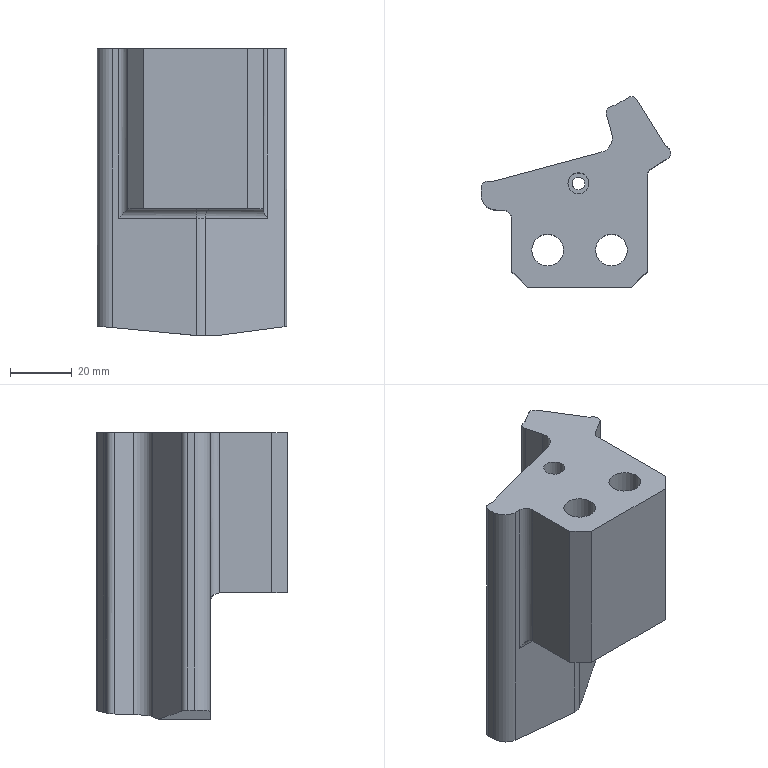Part | NX | features solid 2 | 1 solid | 46 faces | box 61.522 x 61.799 x 92.982 mm | volume 131088 mm3 | cylinder 22 | plane 22 | spline 1 | torus 1 | commonest cylinder face diameters 4 x8 6 x4 10 x4 10.3 x2 17 x2 4.1 x1
STEP:
#1=CARTESIAN_POINT('',(364.121,-6.5,48.));
#2=VERTEX_POINT('',#1);
#3=CARTESIAN_POINT('',(358.971,-6.5,48.));
#4=DIRECTION('',(0.000000738,0.,1.));
#5=DIRECTION('',(1.,0.,-0.000000738));
#6=AXIS2_PLACEMENT_3D('',#3,#4,#5);
#7=CIRCLE('',#6,5.15);
#8=EDGE_CURVE('',#2,#2,#7,.F.);
#9=ORIENTED_EDGE('',*,*,#8,.T.);
#10=EDGE_LOOP('',(#9));
#11=FACE_BOUND('',#10,.T.);
#12=CARTESIAN_POINT('',(353.821,-6.5,78.));
#13=VERTEX_POINT('',#12);
#14=CARTESIAN_POINT('',(358.971,-6.5,78.));
#15=DIRECTION('',(0.,0.,-1.));
#16=DIRECTION('',(-1.,0.,0.));
#17=AXIS2_PLACEMENT_3D('',#14,#15,#16);
#18=CIRCLE('',#17,5.15);
#19=EDGE_CURVE('',#13,#13,#18,.T.);
#20=ORIENTED_EDGE('',*,*,#19,.F.);
#21=EDGE_LOOP('',(#20));
#22=FACE_BOUND('',#21,.T.);
#23=CARTESIAN_POINT('',(358.971,-6.5,54.));
#24=DIRECTION('',(0.000000369,0.000000231,1.));
#25=DIRECTION('',(-1.,0.,0.000000369));
#26=AXIS2_PLACEMENT_3D('',#23,#24,#25);
#27=CYLINDRICAL_SURFACE('',#26,5.15);
#28=ADVANCED_FACE('',(#11,#22),#27,.F.);
#29=ORIENTED_EDGE('',*,*,#8,.F.);
#30=EDGE_LOOP('',(#29));
#31=FACE_BOUND('',#30,.T.);
#32=CARTESIAN_POINT('',(350.471,-6.5,48.));
#33=VERTEX_POINT('',#32);
#34=CARTESIAN_POINT('',(358.971,-6.5,48.));
#35=DIRECTION('',(-0.000000738,0.,-1.));
#36=DIRECTION('',(-1.,0.,0.000000738));
#37=AXIS2_PLACEMENT_3D('',#34,#35,#36);
#38=CIRCLE('',#37,8.5);
#39=EDGE_CURVE('',#33,#33,#38,.T.);
#40=ORIENTED_EDGE('',*,*,#39,.T.);
#41=EDGE_LOOP('',(#40));
#42=FACE_BOUND('',#41,.T.);
#43=CARTESIAN_POINT('',(428.356,-2.,48.));
#44=DIRECTION('',(0.000000738,0.,1.));
#45=DIRECTION('',(1.,0.,-0.000000738));
#46=AXIS2_PLACEMENT_3D('',#43,#44,#45);
#47=PLANE('',#46);
#48=ADVANCED_FACE('',(#31,#42),#47,.F.);
#49=ORIENTED_EDGE('',*,*,#39,.F.);
#50=EDGE_LOOP('',(#49));
#51=FACE_BOUND('',#50,.T.);
#52=CARTESIAN_POINT('',(367.471,-6.5,26.));
#53=VERTEX_POINT('',#52);
#54=CARTESIAN_POINT('',(358.971,-6.5,26.));
#55=DIRECTION('',(0.,0.,1.));
#56=DIRECTION('',(1.,0.,0.));
#57=AXIS2_PLACEMENT_3D('',#54,#55,#56);
#58=CIRCLE('',#57,8.5);
#59=EDGE_CURVE('',#53,#53,#58,.T.);
#60=ORIENTED_EDGE('',*,*,#59,.F.);
#61=EDGE_LOOP('',(#60));
#62=FACE_BOUND('',#61,.T.);
#63=CARTESIAN_POINT('',(358.971,-6.5,19.));
#64=DIRECTION('',(0.000000369,0.000000231,1.));
#65=DIRECTION('',(-1.,0.,0.000000369));
#66=AXIS2_PLACEMENT_3D('',#63,#64,#65);
#67=CYLINDRICAL_SURFACE('',#66,8.5);
#68=ADVANCED_FACE('',(#51,#62),#67,.F.);
#69=CARTESIAN_POINT('',(348.499,17.238,-14.982));
#70=VERTEX_POINT('',#69);
#71=CARTESIAN_POINT('',(348.499,13.166,-14.982));
#72=VERTEX_POINT('',#71);
#73=CARTESIAN_POINT('',(348.26,15.202,-14.982));
#74=DIRECTION('',(-0.000000369,-0.000000231,-1.));
#75=DIRECTION('',(-1.,0.,0.000000369));
#76=AXIS2_PLACEMENT_3D('',#73,#74,#75);
#77=CIRCLE('',#76,2.05);
#78=EDGE_CURVE('',#70,#72,#77,.T.);
#79=ORIENTED_EDGE('',*,*,#78,.F.);
#80=CARTESIAN_POINT('',(348.499,21.837,-14.982));
#81=VERTEX_POINT('',#80);
#82=CARTESIAN_POINT('',(348.499,13.942,-14.982));
#83=DIRECTION('',(0.,1.,-0.000000231));
#84=VECTOR('',#83,1000.);
#85=LINE('',#82,#84);
#86=EDGE_CURVE('',#70,#81,#85,.T.);
#87=ORIENTED_EDGE('',*,*,#86,.T.);
#88=CARTESIAN_POINT('',(355.956,9.904,-14.982));
#89=VERTEX_POINT('',#88);
#90=CARTESIAN_POINT('',(353.665,13.57,-14.982));
#91=DIRECTION('',(0.5299,-0.848,0.));
#92=VECTOR('',#91,1000.);
#93=LINE('',#90,#92);
#94=EDGE_CURVE('',#81,#89,#93,.T.);
#95=ORIENTED_EDGE('',*,*,#94,.T.);
#96=CARTESIAN_POINT('',(351.724,7.26,-14.982));
#97=VERTEX_POINT('',#96);
#98=CARTESIAN_POINT('',(347.525,4.636,-14.982));
#99=DIRECTION('',(0.848,0.5299,-0.000000435));
#100=VECTOR('',#99,1000.);
#101=LINE('',#98,#100);
#102=EDGE_CURVE('',#97,#89,#101,.T.);
#103=ORIENTED_EDGE('',*,*,#102,.F.);
#104=CARTESIAN_POINT('',(349.074,6.5,-14.982));
#105=VERTEX_POINT('',#104);
#106=CARTESIAN_POINT('',(349.074,11.5,-14.982));
#107=DIRECTION('',(-0.000000369,-0.000000231,-1.));
#108=DIRECTION('',(-1.,0.,0.000000369));
#109=AXIS2_PLACEMENT_3D('',#106,#107,#108);
#110=CIRCLE('',#109,5.);
#111=EDGE_CURVE('',#97,#105,#110,.T.);
#112=ORIENTED_EDGE('',*,*,#111,.T.);
#113=CARTESIAN_POINT('',(348.499,6.5,-14.982));
#114=VERTEX_POINT('',#113);
#115=CARTESIAN_POINT('',(297.,6.5,-14.982));
#116=DIRECTION('',(1.,0.,-0.000000369));
#117=VECTOR('',#116,1000.);
#118=LINE('',#115,#117);
#119=EDGE_CURVE('',#114,#105,#118,.T.);
#120=ORIENTED_EDGE('',*,*,#119,.F.);
#121=CARTESIAN_POINT('',(348.499,13.942,-14.982));
#122=DIRECTION('',(0.,1.,-0.000000231));
#123=VECTOR('',#122,1000.);
#124=LINE('',#121,#123);
#125=EDGE_CURVE('',#114,#72,#124,.T.);
#126=ORIENTED_EDGE('',*,*,#125,.T.);
#127=EDGE_LOOP('',(#79,#87,#95,#103,#112,#120,#126));
#128=FACE_BOUND('',#127,.T.);
#129=CARTESIAN_POINT('',(294.129,90.087,-14.982));
#130=DIRECTION('',(-0.000000369,-0.000000231,-1.));
#131=DIRECTION('',(-1.,0.,0.000000369));
#132=AXIS2_PLACEMENT_3D('',#129,#130,#131);
#133=PLANE('',#132);
#134=ADVANCED_FACE('',(#128),#133,.T.);
#135=CARTESIAN_POINT('',(343.413,-6.5,48.));
#136=VERTEX_POINT('',#135);
#137=CARTESIAN_POINT('',(338.263,-6.5,48.));
#138=DIRECTION('',(0.,0.,1.));
#139=DIRECTION('',(1.,0.,0.));
#140=AXIS2_PLACEMENT_3D('',#137,#138,#139);
#141=CIRCLE('',#140,5.15);
#142=EDGE_CURVE('',#136,#136,#141,.F.);
#143=ORIENTED_EDGE('',*,*,#142,.F.);
#144=EDGE_LOOP('',(#143));
#145=FACE_BOUND('',#144,.T.);
#146=CARTESIAN_POINT('',(346.763,-6.5,48.));
#147=VERTEX_POINT('',#146);
#148=CARTESIAN_POINT('',(338.263,-6.5,48.));
#149=DIRECTION('',(0.,0.,1.));
#150=DIRECTION('',(1.,0.,0.));
#151=AXIS2_PLACEMENT_3D('',#148,#149,#150);
#152=CIRCLE('',#151,8.5);
#153=EDGE_CURVE('',#147,#147,#152,.F.);
#154=ORIENTED_EDGE('',*,*,#153,.T.);
#155=EDGE_LOOP('',(#154));
#156=FACE_BOUND('',#155,.T.);
#157=CARTESIAN_POINT('',(268.879,-2.,48.));
#158=DIRECTION('',(0.,0.,1.));
#159=DIRECTION('',(-1.,0.,0.));
#160=AXIS2_PLACEMENT_3D('',#157,#158,#159);
#161=PLANE('',#160);
#162=ADVANCED_FACE('',(#145,#156),#161,.F.);
#163=CARTESIAN_POINT('',(316.719,11.5,-11.955));
#164=VERTEX_POINT('',#163);
#165=CARTESIAN_POINT('',(316.719,11.5,78.));
#166=VERTEX_POINT('',#165);
#167=CARTESIAN_POINT('',(316.719,11.5,-8.));
#168=DIRECTION('',(0.000000369,0.000000231,1.));
#169=VECTOR('',#168,1000.);
#170=LINE('',#167,#169);
#171=EDGE_CURVE('',#164,#166,#170,.T.);
#172=ORIENTED_EDGE('',*,*,#171,.F.);
#173=CARTESIAN_POINT('',(321.719,6.5,-12.431));
#174=VERTEX_POINT('',#173);
#175=CARTESIAN_POINT('',(321.719,11.5,-12.431));
#176=DIRECTION('',(-0.09481,-0.00000023,-0.9955));
#177=DIRECTION('',(-0.9955,0.000000022,0.09481));
#178=AXIS2_PLACEMENT_3D('',#175,#176,#177);
#179=ELLIPSE('',#178,5.023,5.);
#180=EDGE_CURVE('',#164,#174,#179,.F.);
#181=ORIENTED_EDGE('',*,*,#180,.T.);
#182=CARTESIAN_POINT('',(321.719,6.5,78.));
#183=VERTEX_POINT('',#182);
#184=CARTESIAN_POINT('',(321.719,6.5,-8.));
#185=DIRECTION('',(0.000000369,0.000000231,1.));
#186=VECTOR('',#185,1000.);
#187=LINE('',#184,#186);
#188=EDGE_CURVE('',#174,#183,#187,.T.);
#189=ORIENTED_EDGE('',*,*,#188,.T.);
#190=CARTESIAN_POINT('',(321.719,11.5,78.));
#191=DIRECTION('',(0.,0.,-1.));
#192=DIRECTION('',(-1.,0.,0.));
#193=AXIS2_PLACEMENT_3D('',#190,#191,#192);
#194=CIRCLE('',#193,5.);
#195=EDGE_CURVE('',#183,#166,#194,.T.);
#196=ORIENTED_EDGE('',*,*,#195,.T.);
#197=EDGE_LOOP('',(#172,#181,#189,#196));
#198=FACE_BOUND('',#197,.T.);
#199=CARTESIAN_POINT('',(321.719,11.5,-8.));
#200=DIRECTION('',(0.000000369,0.000000231,1.));
#201=DIRECTION('',(1.,0.,-0.000000369));
#202=AXIS2_PLACEMENT_3D('',#199,#200,#201);
#203=CYLINDRICAL_SURFACE('',#202,5.);
#204=ADVANCED_FACE('',(#198),#203,.T.);
#205=CARTESIAN_POINT('',(316.719,13.767,-11.955));
#206=VERTEX_POINT('',#205);
#207=CARTESIAN_POINT('',(316.719,13.767,78.));
#208=VERTEX_POINT('',#207);
#209=CARTESIAN_POINT('',(316.719,13.767,-8.));
#210=DIRECTION('',(0.000000369,0.000000231,1.));
#211=VECTOR('',#210,1000.);
#212=LINE('',#209,#211);
#213=EDGE_CURVE('',#206,#208,#212,.T.);
#214=ORIENTED_EDGE('',*,*,#213,.F.);
#215=CARTESIAN_POINT('',(316.719,90.087,-11.955));
#216=DIRECTION('',(0.,-1.,0.000000231));
#217=VECTOR('',#216,1000.);
#218=LINE('',#215,#217);
#219=EDGE_CURVE('',#206,#164,#218,.T.);
#220=ORIENTED_EDGE('',*,*,#219,.T.);
#221=ORIENTED_EDGE('',*,*,#171,.T.);
#222=CARTESIAN_POINT('',(316.719,89.912,78.));
#223=DIRECTION('',(0.,1.,0.));
#224=VECTOR('',#223,1000.);
#225=LINE('',#222,#224);
#226=EDGE_CURVE('',#166,#208,#225,.T.);
#227=ORIENTED_EDGE('',*,*,#226,.T.);
#228=EDGE_LOOP('',(#214,#220,#221,#227));
#229=FACE_BOUND('',#228,.T.);
#230=CARTESIAN_POINT('',(316.719,89.912,-8.));
#231=DIRECTION('',(1.,0.,-0.000000369));
#232=DIRECTION('',(-0.000000369,0.,-1.));
#233=AXIS2_PLACEMENT_3D('',#230,#231,#232);
#234=PLANE('',#233);
#235=ADVANCED_FACE('',(#229),#234,.F.);
#236=CARTESIAN_POINT('',(318.201,15.698,-12.096));
#237=VERTEX_POINT('',#236);
#238=CARTESIAN_POINT('',(318.201,15.698,78.));
#239=VERTEX_POINT('',#238);
#240=CARTESIAN_POINT('',(318.201,15.698,-8.));
#241=DIRECTION('',(0.000000369,0.000000231,1.));
#242=VECTOR('',#241,1000.);
#243=LINE('',#240,#242);
#244=EDGE_CURVE('',#237,#239,#243,.T.);
#245=ORIENTED_EDGE('',*,*,#244,.F.);
#246=CARTESIAN_POINT('',(318.719,13.767,-12.145));
#247=DIRECTION('',(-0.09481,-0.00000023,-0.9955));
#248=DIRECTION('',(-0.9955,0.000000022,0.09481));
#249=AXIS2_PLACEMENT_3D('',#246,#247,#248);
#250=ELLIPSE('',#249,2.009,2.);
#251=EDGE_CURVE('',#237,#206,#250,.F.);
#252=ORIENTED_EDGE('',*,*,#251,.T.);
#253=ORIENTED_EDGE('',*,*,#213,.T.);
#254=CARTESIAN_POINT('',(318.719,13.767,78.));
#255=DIRECTION('',(0.,0.,-1.));
#256=DIRECTION('',(-1.,0.,0.));
#257=AXIS2_PLACEMENT_3D('',#254,#255,#256);
#258=CIRCLE('',#257,2.);
#259=EDGE_CURVE('',#208,#239,#258,.T.);
#260=ORIENTED_EDGE('',*,*,#259,.T.);
#261=EDGE_LOOP('',(#245,#252,#253,#260));
#262=FACE_BOUND('',#261,.T.);
#263=CARTESIAN_POINT('',(318.719,13.767,-8.));
#264=DIRECTION('',(0.000000369,0.000000231,1.));
#265=DIRECTION('',(1.,0.,-0.000000369));
#266=AXIS2_PLACEMENT_3D('',#263,#264,#265);
#267=CYLINDRICAL_SURFACE('',#266,2.);
#268=ADVANCED_FACE('',(#262),#267,.T.);
#269=CARTESIAN_POINT('',(318.626,15.812,-12.137));
#270=VERTEX_POINT('',#269);
#271=CARTESIAN_POINT('',(318.626,15.812,78.));
#272=VERTEX_POINT('',#271);
#273=CARTESIAN_POINT('',(318.626,15.812,-8.));
#274=DIRECTION('',(0.000000369,0.000000231,1.));
#275=VECTOR('',#274,1000.);
#276=LINE('',#273,#275);
#277=EDGE_CURVE('',#270,#272,#276,.T.);
#278=ORIENTED_EDGE('',*,*,#277,.F.);
#279=CARTESIAN_POINT('',(364.928,28.219,-16.546));
#280=DIRECTION('',(-0.9619,-0.2577,0.09161));
#281=VECTOR('',#280,1000.);
#282=LINE('',#279,#281);
#283=EDGE_CURVE('',#270,#237,#282,.T.);
#284=ORIENTED_EDGE('',*,*,#283,.T.);
#285=ORIENTED_EDGE('',*,*,#244,.T.);
#286=CARTESIAN_POINT('',(303.806,11.841,78.));
#287=DIRECTION('',(0.9659,0.2588,0.));
#288=VECTOR('',#287,1000.);
#289=LINE('',#286,#288);
#290=EDGE_CURVE('',#239,#272,#289,.T.);
#291=ORIENTED_EDGE('',*,*,#290,.T.);
#292=EDGE_LOOP('',(#278,#284,#285,#291));
#293=FACE_BOUND('',#292,.T.);
#294=CARTESIAN_POINT('',(303.806,11.841,-8.));
#295=DIRECTION('',(0.2588,-0.9659,0.000000127));
#296=DIRECTION('',(0.9659,0.2588,0.));
#297=AXIS2_PLACEMENT_3D('',#294,#295,#296);
#298=PLANE('',#297);
#299=ADVANCED_FACE('',(#293),#298,.F.);
#300=CARTESIAN_POINT('',(319.626,15.821,-12.232));
#301=VERTEX_POINT('',#300);
#302=CARTESIAN_POINT('',(319.626,15.821,78.));
#303=VERTEX_POINT('',#302);
#304=CARTESIAN_POINT('',(319.626,15.821,-8.));
#305=DIRECTION('',(0.000000369,0.000000231,1.));
#306=VECTOR('',#305,1000.);
#307=LINE('',#304,#306);
#308=EDGE_CURVE('',#301,#303,#307,.T.);
#309=ORIENTED_EDGE('',*,*,#308,.F.);
#310=CARTESIAN_POINT('',(319.143,13.88,-12.186));
#311=DIRECTION('',(-0.09481,-0.00000023,-0.9955));
#312=DIRECTION('',(-0.9955,0.000000022,0.09481));
#313=AXIS2_PLACEMENT_3D('',#310,#311,#312);
#314=ELLIPSE('',#313,2.009,2.);
#315=EDGE_CURVE('',#301,#270,#314,.F.);
#316=ORIENTED_EDGE('',*,*,#315,.T.);
#317=ORIENTED_EDGE('',*,*,#277,.T.);
#318=CARTESIAN_POINT('',(319.143,13.88,78.));
#319=DIRECTION('',(0.,0.,-1.));
#320=DIRECTION('',(-1.,0.,0.));
#321=AXIS2_PLACEMENT_3D('',#318,#319,#320);
#322=CIRCLE('',#321,2.);
#323=EDGE_CURVE('',#272,#303,#322,.T.);
#324=ORIENTED_EDGE('',*,*,#323,.T.);
#325=EDGE_LOOP('',(#309,#316,#317,#324));
#326=FACE_BOUND('',#325,.T.);
#327=CARTESIAN_POINT('',(319.143,13.88,-8.));
#328=DIRECTION('',(0.000000369,0.000000231,1.));
#329=DIRECTION('',(1.,0.,-0.000000369));
#330=AXIS2_PLACEMENT_3D('',#327,#328,#329);
#331=CYLINDRICAL_SURFACE('',#330,2.);
#332=ADVANCED_FACE('',(#326),#331,.T.);
#333=CARTESIAN_POINT('',(320.626,15.83,-12.327));
#334=VERTEX_POINT('',#333);
#335=CARTESIAN_POINT('',(320.626,15.831,78.));
#336=VERTEX_POINT('',#335);
#337=CARTESIAN_POINT('',(320.626,15.83,-8.));
#338=DIRECTION('',(0.000000369,0.000000231,1.));
#339=VECTOR('',#338,1000.);
#340=LINE('',#337,#339);
#341=EDGE_CURVE('',#334,#336,#340,.T.);
#342=ORIENTED_EDGE('',*,*,#341,.F.);
#343=CARTESIAN_POINT('',(320.108,17.762,-12.278));
#344=DIRECTION('',(-0.09481,-0.00000023,-0.9955));
#345=DIRECTION('',(-0.9955,0.000000022,0.09481));
#346=AXIS2_PLACEMENT_3D('',#343,#344,#345);
#347=ELLIPSE('',#346,2.009,2.);
#348=EDGE_CURVE('',#334,#301,#347,.T.);
#349=ORIENTED_EDGE('',*,*,#348,.T.);
#350=ORIENTED_EDGE('',*,*,#308,.T.);
#351=CARTESIAN_POINT('',(320.108,17.762,78.));
#352=DIRECTION('',(0.,0.,-1.));
#353=DIRECTION('',(-1.,0.,0.));
#354=AXIS2_PLACEMENT_3D('',#351,#352,#353);
#355=CIRCLE('',#354,2.);
#356=EDGE_CURVE('',#303,#336,#355,.F.);
#357=ORIENTED_EDGE('',*,*,#356,.T.);
#358=EDGE_LOOP('',(#342,#349,#350,#357));
#359=FACE_BOUND('',#358,.T.);
#360=CARTESIAN_POINT('',(320.108,17.762,-8.));
#361=DIRECTION('',(0.000000369,0.000000231,1.));
#362=DIRECTION('',(1.,0.,-0.000000369));
#363=AXIS2_PLACEMENT_3D('',#360,#361,#362);
#364=CYLINDRICAL_SURFACE('',#363,2.);
#365=ADVANCED_FACE('',(#359),#364,.F.);
#366=CARTESIAN_POINT('',(355.551,25.189,-14.12));
#367=VERTEX_POINT('',#366);
#368=CARTESIAN_POINT('',(348.08,23.187,-14.942));
#369=VERTEX_POINT('',#368);
#370=CARTESIAN_POINT('',(323.92,16.713,-17.599));
#371=DIRECTION('',(-0.9605,-0.2574,-0.1057));
#372=VECTOR('',#371,1000.);
#373=LINE('',#370,#372);
#374=EDGE_CURVE('',#367,#369,#373,.T.);
#375=ORIENTED_EDGE('',*,*,#374,.T.);
#376=CARTESIAN_POINT('',(365.056,27.736,-16.559));
#377=DIRECTION('',(-0.9619,-0.2577,0.09161));
#378=VECTOR('',#377,1000.);
#379=LINE('',#376,#378);
#380=EDGE_CURVE('',#369,#334,#379,.T.);
#381=ORIENTED_EDGE('',*,*,#380,.T.);
#382=ORIENTED_EDGE('',*,*,#341,.T.);
#383=CARTESIAN_POINT('',(355.551,25.189,78.));
#384=VERTEX_POINT('',#383);
#385=CARTESIAN_POINT('',(320.626,15.831,78.));
#386=DIRECTION('',(0.9659,0.2588,0.));
#387=VECTOR('',#386,1000.);
#388=LINE('',#385,#387);
#389=EDGE_CURVE('',#336,#384,#388,.T.);
#390=ORIENTED_EDGE('',*,*,#389,.T.);
#391=CARTESIAN_POINT('',(355.551,25.189,-8.));
#392=DIRECTION('',(0.000000369,0.000000231,1.));
#393=VECTOR('',#392,1000.);
#394=LINE('',#391,#393);
#395=EDGE_CURVE('',#367,#384,#394,.T.);
#396=ORIENTED_EDGE('',*,*,#395,.F.);
#397=EDGE_LOOP('',(#375,#381,#382,#390,#396));
#398=FACE_BOUND('',#397,.T.);
#399=CARTESIAN_POINT('',(320.626,15.83,-8.));
#400=DIRECTION('',(0.2588,-0.9659,0.000000127));
#401=DIRECTION('',(0.9659,0.2588,0.));
#402=AXIS2_PLACEMENT_3D('',#399,#400,#401);
#403=PLANE('',#402);
#404=ADVANCED_FACE('',(#398),#403,.F.);
#405=CARTESIAN_POINT('',(359.061,31.404,-13.423));
#406=VERTEX_POINT('',#405);
#407=CARTESIAN_POINT('',(359.061,31.404,78.));
#408=VERTEX_POINT('',#407);
#409=CARTESIAN_POINT('',(359.061,31.404,-8.));
#410=DIRECTION('',(0.000000369,0.000000231,1.));
#411=VECTOR('',#410,1000.);
#412=LINE('',#409,#411);
#413=EDGE_CURVE('',#406,#408,#412,.T.);
#414=ORIENTED_EDGE('',*,*,#413,.F.);
#415=CARTESIAN_POINT('',(354.257,30.018,-13.957));
#416=DIRECTION('',(0.09365,0.05852,-0.9939));
#417=DIRECTION('',(0.8429,0.5267,0.1104));
#418=AXIS2_PLACEMENT_3D('',#415,#416,#417);
#419=ELLIPSE('',#418,5.031,5.);
#420=EDGE_CURVE('',#406,#367,#419,.T.);
#421=ORIENTED_EDGE('',*,*,#420,.T.);
#422=ORIENTED_EDGE('',*,*,#395,.T.);
#423=CARTESIAN_POINT('',(354.257,30.018,78.));
#424=DIRECTION('',(0.,0.,-1.));
#425=DIRECTION('',(-1.,0.,0.));
#426=AXIS2_PLACEMENT_3D('',#423,#424,#425);
#427=CIRCLE('',#426,5.);
#428=EDGE_CURVE('',#384,#408,#427,.F.);
#429=ORIENTED_EDGE('',*,*,#428,.T.);
#430=EDGE_LOOP('',(#414,#421,#422,#429));
#431=FACE_BOUND('',#430,.T.);
#432=CARTESIAN_POINT('',(354.257,30.018,-8.));
#433=DIRECTION('',(0.000000369,0.000000231,1.));
#434=DIRECTION('',(1.,0.,-0.000000369));
#435=AXIS2_PLACEMENT_3D('',#432,#433,#434);
#436=CYLINDRICAL_SURFACE('',#435,5.);
#437=ADVANCED_FACE('',(#431),#436,.F.);
#438=CARTESIAN_POINT('',(357.296,37.575,78.));
#439=VERTEX_POINT('',#438);
#440=CARTESIAN_POINT('',(357.296,37.575,-13.226));
#441=VERTEX_POINT('',#440);
#442=CARTESIAN_POINT('',(357.296,37.575,82.));
#443=DIRECTION('',(0.000000369,0.000000231,1.));
#444=VECTOR('',#443,1000.);
#445=LINE('',#442,#444);
#446=EDGE_CURVE('',#439,#441,#445,.F.);
#447=ORIENTED_EDGE('',*,*,#446,.T.);
#448=CARTESIAN_POINT('',(357.296,37.575,-13.226));
#449=CARTESIAN_POINT('',(357.879,35.516,-13.292));
#450=CARTESIAN_POINT('',(358.468,33.46,-13.358));
#451=CARTESIAN_POINT('',(359.061,31.404,-13.423));
#452=B_SPLINE_CURVE_WITH_KNOTS('',3,(#448,#449,#450,#451),.UNSPECIFIED.,.F.,.F.,(4,4),(0.,0.006421),.UNSPECIFIED.);
#453=EDGE_CURVE('',#441,#406,#452,.T.);
#454=ORIENTED_EDGE('',*,*,#453,.T.);
#455=ORIENTED_EDGE('',*,*,#413,.T.);
#456=CARTESIAN_POINT('',(359.061,31.404,78.));
#457=CARTESIAN_POINT('',(358.469,33.46,78.));
#458=CARTESIAN_POINT('',(357.879,35.516,78.));
#459=CARTESIAN_POINT('',(357.296,37.575,78.));
#460=B_SPLINE_CURVE_WITH_KNOTS('',3,(#456,#457,#458,#459),.UNSPECIFIED.,.F.,.F.,(4,4),(0.,0.006418),.UNSPECIFIED.);
#461=EDGE_CURVE('',#408,#439,#460,.T.);
#462=ORIENTED_EDGE('',*,*,#461,.T.);
#463=EDGE_LOOP('',(#447,#454,#455,#462));
#464=FACE_BOUND('',#463,.T.);
#465=CARTESIAN_POINT('',(359.061,31.404,-13.972));
#466=CARTESIAN_POINT('',(359.061,31.404,78.));
#467=CARTESIAN_POINT('',(358.468,33.46,-13.972));
#468=CARTESIAN_POINT('',(358.469,33.46,78.));
#469=CARTESIAN_POINT('',(357.879,35.516,-13.972));
#470=CARTESIAN_POINT('',(357.879,35.516,78.));
#471=CARTESIAN_POINT('',(357.296,37.575,-13.972));
#472=CARTESIAN_POINT('',(357.296,37.575,78.));
#473=B_SPLINE_SURFACE_WITH_KNOTS('',3,1,((#465,#466),(#467,#468),(#469,#470),(#471,#472)),.SURF_OF_LINEAR_EXTRUSION.,.F.,.F.,.F.,(4,4),(2,2),(-0.02584,0.4694),(0.,1.),.PIECEWISE_BEZIER_KNOTS.);
#474=ADVANCED_FACE('',(#464),#473,.F.);
#475=CARTESIAN_POINT('',(358.674,40.044,-12.951));
#476=VERTEX_POINT('',#475);
#477=CARTESIAN_POINT('',(358.674,40.044,78.));
#478=VERTEX_POINT('',#477);
#479=CARTESIAN_POINT('',(358.674,40.044,82.));
#480=DIRECTION('',(-0.000000369,-0.000000231,-1.));
#481=VECTOR('',#480,1000.);
#482=LINE('',#479,#481);
#483=EDGE_CURVE('',#476,#478,#482,.F.);
#484=ORIENTED_EDGE('',*,*,#483,.F.);
#485=CARTESIAN_POINT('',(359.22,38.12,-13.013));
#486=DIRECTION('',(0.09365,0.05852,-0.9939));
#487=DIRECTION('',(0.8429,0.5267,0.1104));
#488=AXIS2_PLACEMENT_3D('',#485,#486,#487);
#489=ELLIPSE('',#488,2.012,2.);
#490=EDGE_CURVE('',#476,#441,#489,.F.);
#491=ORIENTED_EDGE('',*,*,#490,.T.);
#492=ORIENTED_EDGE('',*,*,#446,.F.);
#493=CARTESIAN_POINT('',(359.22,38.12,78.));
#494=DIRECTION('',(0.,0.,-1.));
#495=DIRECTION('',(-1.,0.,0.));
#496=AXIS2_PLACEMENT_3D('',#493,#494,#495);
#497=CIRCLE('',#496,2.);
#498=EDGE_CURVE('',#478,#439,#497,.F.);
#499=ORIENTED_EDGE('',*,*,#498,.F.);
#500=EDGE_LOOP('',(#484,#491,#492,#499));
#501=FACE_BOUND('',#500,.T.);
#502=CARTESIAN_POINT('',(359.22,38.12,37.));
#503=DIRECTION('',(0.000000369,0.000000231,1.));
#504=DIRECTION('',(1.,0.,-0.000000369));
#505=AXIS2_PLACEMENT_3D('',#502,#503,#504);
#506=CYLINDRICAL_SURFACE('',#505,2.);
#507=ADVANCED_FACE('',(#501),#506,.T.);
#508=CARTESIAN_POINT('',(359.771,40.356,78.));
#509=VERTEX_POINT('',#508);
#510=CARTESIAN_POINT('',(359.771,40.356,-12.829));
#511=VERTEX_POINT('',#510);
#512=CARTESIAN_POINT('',(359.771,40.356,-8.));
#513=DIRECTION('',(0.000000369,0.000000231,1.));
#514=VECTOR('',#513,1000.);
#515=LINE('',#512,#514);
#516=EDGE_CURVE('',#509,#511,#515,.F.);
#517=ORIENTED_EDGE('',*,*,#516,.T.);
#518=CARTESIAN_POINT('',(312.387,26.918,-18.085));
#519=DIRECTION('',(-0.9566,-0.2713,-0.1061));
#520=VECTOR('',#519,1000.);
#521=LINE('',#518,#520);
#522=EDGE_CURVE('',#511,#476,#521,.T.);
#523=ORIENTED_EDGE('',*,*,#522,.T.);
#524=ORIENTED_EDGE('',*,*,#483,.T.);
#525=CARTESIAN_POINT('',(311.762,26.741,78.));
#526=DIRECTION('',(-0.9621,-0.2728,0.));
#527=VECTOR('',#526,1000.);
#528=LINE('',#525,#527);
#529=EDGE_CURVE('',#509,#478,#528,.T.);
#530=ORIENTED_EDGE('',*,*,#529,.F.);
#531=EDGE_LOOP('',(#517,#523,#524,#530));
#532=FACE_BOUND('',#531,.T.);
#533=CARTESIAN_POINT('',(311.762,26.741,-8.));
#534=DIRECTION('',(-0.2728,0.9621,-0.000000121));
#535=DIRECTION('',(-0.9621,-0.2728,0.));
#536=AXIS2_PLACEMENT_3D('',#533,#534,#535);
#537=PLANE('',#536);
#538=ADVANCED_FACE('',(#532),#537,.T.);
#539=CARTESIAN_POINT('',(361.056,40.926,-12.675));
#540=VERTEX_POINT('',#539);
#541=CARTESIAN_POINT('',(361.057,40.926,78.));
#542=VERTEX_POINT('',#541);
#543=CARTESIAN_POINT('',(361.057,40.926,82.));
#544=DIRECTION('',(0.000000369,0.000000231,1.));
#545=VECTOR('',#544,1000.);
#546=LINE('',#543,#545);
#547=EDGE_CURVE('',#540,#542,#546,.T.);
#548=ORIENTED_EDGE('',*,*,#547,.F.);
#549=CARTESIAN_POINT('',(358.407,45.166,-12.675));
#550=DIRECTION('',(0.09365,0.05852,-0.9939));
#551=DIRECTION('',(-0.8429,-0.5267,-0.1104));
#552=AXIS2_PLACEMENT_3D('',#549,#550,#551);
#553=ELLIPSE('',#552,5.031,5.);
#554=EDGE_CURVE('',#540,#511,#553,.T.);
#555=ORIENTED_EDGE('',*,*,#554,.T.);
#556=ORIENTED_EDGE('',*,*,#516,.F.);
#557=CARTESIAN_POINT('',(358.407,45.166,78.));
#558=DIRECTION('',(0.,0.,-1.));
#559=DIRECTION('',(-1.,0.,0.));
#560=AXIS2_PLACEMENT_3D('',#557,#558,#559);
#561=CIRCLE('',#560,5.);
#562=EDGE_CURVE('',#542,#509,#561,.T.);
#563=ORIENTED_EDGE('',*,*,#562,.F.);
#564=EDGE_LOOP('',(#548,#555,#556,#563));
#565=FACE_BOUND('',#564,.T.);
#566=CARTESIAN_POINT('',(358.407,45.166,-8.));
#567=DIRECTION('',(-0.000000369,-0.000000231,-1.));
#568=DIRECTION('',(-1.,0.,0.000000369));
#569=AXIS2_PLACEMENT_3D('',#566,#567,#568);
#570=CYLINDRICAL_SURFACE('',#569,5.);
#571=ADVANCED_FACE('',(#565),#570,.F.);
#572=CARTESIAN_POINT('',(364.368,42.995,78.));
#573=VERTEX_POINT('',#572);
#574=CARTESIAN_POINT('',(364.368,42.995,-12.241));
#575=VERTEX_POINT('',#574);
#576=CARTESIAN_POINT('',(364.368,42.995,-8.));
#577=DIRECTION('',(-0.000000369,-0.000000231,-1.));
#578=VECTOR('',#577,1000.);
#579=LINE('',#576,#578);
#580=EDGE_CURVE('',#573,#575,#579,.T.);
#581=ORIENTED_EDGE('',*,*,#580,.T.);
#582=CARTESIAN_POINT('',(335.119,24.718,-16.073));
#583=DIRECTION('',(-0.8429,-0.5267,-0.1104));
#584=VECTOR('',#583,1000.);
#585=LINE('',#582,#584);
#586=EDGE_CURVE('',#575,#540,#585,.T.);
#587=ORIENTED_EDGE('',*,*,#586,.T.);
#588=ORIENTED_EDGE('',*,*,#547,.T.);
#589=CARTESIAN_POINT('',(334.735,24.478,78.));
#590=DIRECTION('',(-0.848,-0.5299,0.));
#591=VECTOR('',#590,1000.);
#592=LINE('',#589,#591);
#593=EDGE_CURVE('',#573,#542,#592,.T.);
#594=ORIENTED_EDGE('',*,*,#593,.F.);
#595=EDGE_LOOP('',(#581,#587,#588,#594));
#596=FACE_BOUND('',#595,.T.);
#597=CARTESIAN_POINT('',(334.735,24.478,-8.));
#598=DIRECTION('',(-0.5299,0.848,0.));
#599=DIRECTION('',(-0.848,-0.5299,0.));
#600=AXIS2_PLACEMENT_3D('',#597,#598,#599);
#601=PLANE('',#600);
#602=ADVANCED_FACE('',(#596),#601,.T.);
#603=CARTESIAN_POINT('',(367.124,42.358,-12.018));
#604=VERTEX_POINT('',#603);
#605=CARTESIAN_POINT('',(367.124,42.358,78.));
#606=VERTEX_POINT('',#605);
#607=CARTESIAN_POINT('',(367.124,42.358,82.));
#608=DIRECTION('',(-0.000000369,-0.000000231,-1.));
#609=VECTOR('',#608,1000.);
#610=LINE('',#607,#609);
#611=EDGE_CURVE('',#604,#606,#610,.F.);
#612=ORIENTED_EDGE('',*,*,#611,.F.);
#613=CARTESIAN_POINT('',(365.427,41.299,-12.241));
#614=DIRECTION('',(0.09365,0.05852,-0.9939));
#615=DIRECTION('',(0.8429,0.5267,0.1104));
#616=AXIS2_PLACEMENT_3D('',#613,#614,#615);
#617=ELLIPSE('',#616,2.012,2.);
#618=EDGE_CURVE('',#604,#575,#617,.F.);
#619=ORIENTED_EDGE('',*,*,#618,.T.);
#620=ORIENTED_EDGE('',*,*,#580,.F.);
#621=CARTESIAN_POINT('',(365.428,41.299,78.));
#622=DIRECTION('',(0.,0.,-1.));
#623=DIRECTION('',(-1.,0.,0.));
#624=AXIS2_PLACEMENT_3D('',#621,#622,#623);
#625=CIRCLE('',#624,2.);
#626=EDGE_CURVE('',#606,#573,#625,.F.);
#627=ORIENTED_EDGE('',*,*,#626,.F.);
#628=EDGE_LOOP('',(#612,#619,#620,#627));
#629=FACE_BOUND('',#628,.T.);
#630=CARTESIAN_POINT('',(365.427,41.299,-8.));
#631=DIRECTION('',(0.000000369,0.000000231,1.));
#632=DIRECTION('',(1.,0.,-0.000000369));
#633=AXIS2_PLACEMENT_3D('',#630,#631,#632);
#634=CYLINDRICAL_SURFACE('',#633,2.);
#635=ADVANCED_FACE('',(#629),#634,.T.);
#636=CARTESIAN_POINT('',(376.282,27.703,-12.018));
#637=VERTEX_POINT('',#636);
#638=CARTESIAN_POINT('',(376.282,27.703,78.));
#639=VERTEX_POINT('',#638);
#640=CARTESIAN_POINT('',(376.282,27.703,-8.));
#641=DIRECTION('',(0.000000369,0.000000231,1.));
#642=VECTOR('',#641,1000.);
#643=LINE('',#640,#642);
#644=EDGE_CURVE('',#637,#639,#643,.T.);
#645=ORIENTED_EDGE('',*,*,#644,.F.);
#646=CARTESIAN_POINT('',(325.176,109.488,-12.018));
#647=DIRECTION('',(-0.5299,0.848,0.));
#648=VECTOR('',#647,1000.);
#649=LINE('',#646,#648);
#650=EDGE_CURVE('',#637,#604,#649,.T.);
#651=ORIENTED_EDGE('',*,*,#650,.T.);
#652=ORIENTED_EDGE('',*,*,#611,.T.);
#653=CARTESIAN_POINT('',(367.124,42.358,78.));
#654=DIRECTION('',(0.5299,-0.848,0.));
#655=VECTOR('',#654,1000.);
#656=LINE('',#653,#655);
#657=EDGE_CURVE('',#606,#639,#656,.T.);
#658=ORIENTED_EDGE('',*,*,#657,.T.);
#659=EDGE_LOOP('',(#645,#651,#652,#658));
#660=FACE_BOUND('',#659,.T.);
#661=CARTESIAN_POINT('',(367.124,42.358,-8.));
#662=DIRECTION('',(-0.848,-0.5299,0.000000435));
#663=DIRECTION('',(0.5299,-0.848,0.));
#664=AXIS2_PLACEMENT_3D('',#661,#662,#663);
#665=PLANE('',#664);
#666=ADVANCED_FACE('',(#660),#665,.F.);
#667=CARTESIAN_POINT('',(377.007,27.014,-11.991));
#668=VERTEX_POINT('',#667);
#669=CARTESIAN_POINT('',(377.007,27.014,78.));
#670=VERTEX_POINT('',#669);
#671=CARTESIAN_POINT('',(377.007,27.014,-8.));
#672=DIRECTION('',(0.000000369,0.000000231,1.));
#673=VECTOR('',#672,1000.);
#674=LINE('',#671,#673);
#675=EDGE_CURVE('',#668,#670,#674,.T.);
#676=ORIENTED_EDGE('',*,*,#675,.F.);
#677=CARTESIAN_POINT('',(377.978,28.762,-11.796));
#678=DIRECTION('',(0.09365,0.05852,-0.9939));
#679=DIRECTION('',(0.8429,0.5267,0.1104));
#680=AXIS2_PLACEMENT_3D('',#677,#678,#679);
#681=ELLIPSE('',#680,2.012,2.);
#682=EDGE_CURVE('',#668,#637,#681,.T.);
#683=ORIENTED_EDGE('',*,*,#682,.T.);
#684=ORIENTED_EDGE('',*,*,#644,.T.);
#685=CARTESIAN_POINT('',(377.978,28.763,78.));
#686=DIRECTION('',(0.,0.,-1.));
#687=DIRECTION('',(-1.,0.,0.));
#688=AXIS2_PLACEMENT_3D('',#685,#686,#687);
#689=CIRCLE('',#688,2.);
#690=EDGE_CURVE('',#639,#670,#689,.F.);
#691=ORIENTED_EDGE('',*,*,#690,.T.);
#692=EDGE_LOOP('',(#676,#683,#684,#691));
#693=FACE_BOUND('',#692,.T.);
#694=CARTESIAN_POINT('',(377.978,28.762,-8.));
#695=DIRECTION('',(0.000000369,0.000000231,1.));
#696=DIRECTION('',(1.,0.,-0.000000369));
#697=AXIS2_PLACEMENT_3D('',#694,#695,#696);
#698=CYLINDRICAL_SURFACE('',#697,2.);
#699=ADVANCED_FACE('',(#693),#698,.F.);
#700=CARTESIAN_POINT('',(377.732,26.325,-11.963));
#701=VERTEX_POINT('',#700);
#702=CARTESIAN_POINT('',(377.732,26.325,78.));
#703=VERTEX_POINT('',#702);
#704=CARTESIAN_POINT('',(377.732,26.325,-8.));
#705=DIRECTION('',(0.000000369,0.000000231,1.));
#706=VECTOR('',#705,1000.);
#707=LINE('',#704,#706);
#708=EDGE_CURVE('',#701,#703,#707,.T.);
#709=ORIENTED_EDGE('',*,*,#708,.F.);
#710=CARTESIAN_POINT('',(376.036,25.266,-12.185));
#711=DIRECTION('',(0.09365,0.05852,-0.9939));
#712=DIRECTION('',(0.8429,0.5267,0.1104));
#713=AXIS2_PLACEMENT_3D('',#710,#711,#712);
#714=ELLIPSE('',#713,2.012,2.);
#715=EDGE_CURVE('',#701,#668,#714,.F.);
#716=ORIENTED_EDGE('',*,*,#715,.T.);
#717=ORIENTED_EDGE('',*,*,#675,.T.);
#718=CARTESIAN_POINT('',(376.036,25.266,78.));
#719=DIRECTION('',(0.,0.,-1.));
#720=DIRECTION('',(-1.,0.,0.));
#721=AXIS2_PLACEMENT_3D('',#718,#719,#720);
#722=CIRCLE('',#721,2.);
#723=EDGE_CURVE('',#670,#703,#722,.T.);
#724=ORIENTED_EDGE('',*,*,#723,.T.);
#725=EDGE_LOOP('',(#709,#716,#717,#724));
#726=FACE_BOUND('',#725,.T.);
#727=CARTESIAN_POINT('',(376.036,25.266,-8.));
#728=DIRECTION('',(0.000000369,0.000000231,1.));
#729=DIRECTION('',(1.,0.,-0.000000369));
#730=AXIS2_PLACEMENT_3D('',#727,#728,#729);
#731=CYLINDRICAL_SURFACE('',#730,2.);
#732=ADVANCED_FACE('',(#726),#731,.T.);
#733=CARTESIAN_POINT('',(377.936,25.998,-11.963));
#734=VERTEX_POINT('',#733);
#735=CARTESIAN_POINT('',(377.937,25.998,78.));
#736=VERTEX_POINT('',#735);
#737=CARTESIAN_POINT('',(377.936,25.998,-8.));
#738=DIRECTION('',(0.000000369,0.000000231,1.));
#739=VECTOR('',#738,1000.);
#740=LINE('',#737,#739);
#741=EDGE_CURVE('',#734,#736,#740,.T.);
#742=ORIENTED_EDGE('',*,*,#741,.F.);
#743=CARTESIAN_POINT('',(325.6,109.753,-11.963));
#744=DIRECTION('',(-0.5299,0.848,0.));
#745=VECTOR('',#744,1000.);
#746=LINE('',#743,#745);
#747=EDGE_CURVE('',#734,#701,#746,.T.);
#748=ORIENTED_EDGE('',*,*,#747,.T.);
#749=ORIENTED_EDGE('',*,*,#708,.T.);
#750=CARTESIAN_POINT('',(375.858,29.324,78.));
#751=DIRECTION('',(0.5299,-0.848,0.));
#752=VECTOR('',#751,1000.);
#753=LINE('',#750,#752);
#754=EDGE_CURVE('',#703,#736,#753,.T.);
#755=ORIENTED_EDGE('',*,*,#754,.T.);
#756=EDGE_LOOP('',(#742,#748,#749,#755));
#757=FACE_BOUND('',#756,.T.);
#758=CARTESIAN_POINT('',(375.858,29.324,-8.));
#759=DIRECTION('',(-0.848,-0.5299,0.000000435));
#760=DIRECTION('',(0.5299,-0.848,0.));
#761=AXIS2_PLACEMENT_3D('',#758,#759,#760);
#762=PLANE('',#761);
#763=ADVANCED_FACE('',(#757),#762,.F.);
#764=CARTESIAN_POINT('',(377.3,23.242,-12.185));
#765=VERTEX_POINT('',#764);
#766=CARTESIAN_POINT('',(377.3,23.242,78.));
#767=VERTEX_POINT('',#766);
#768=CARTESIAN_POINT('',(377.3,23.242,-8.));
#769=DIRECTION('',(0.000000369,0.000000231,1.));
#770=VECTOR('',#769,1000.);
#771=LINE('',#768,#770);
#772=EDGE_CURVE('',#765,#767,#771,.T.);
#773=ORIENTED_EDGE('',*,*,#772,.F.);
#774=CARTESIAN_POINT('',(376.24,24.938,-12.185));
#775=DIRECTION('',(0.09365,0.05852,-0.9939));
#776=DIRECTION('',(0.8429,0.5267,0.1104));
#777=AXIS2_PLACEMENT_3D('',#774,#775,#776);
#778=ELLIPSE('',#777,2.012,2.);
#779=EDGE_CURVE('',#765,#734,#778,.F.);
#780=ORIENTED_EDGE('',*,*,#779,.T.);
#781=ORIENTED_EDGE('',*,*,#741,.T.);
#782=CARTESIAN_POINT('',(376.24,24.938,78.));
#783=DIRECTION('',(0.,0.,-1.));
#784=DIRECTION('',(-1.,0.,0.));
#785=AXIS2_PLACEMENT_3D('',#782,#783,#784);
#786=CIRCLE('',#785,2.);
#787=EDGE_CURVE('',#736,#767,#786,.T.);
#788=ORIENTED_EDGE('',*,*,#787,.T.);
#789=EDGE_LOOP('',(#773,#780,#781,#788));
#790=FACE_BOUND('',#789,.T.);
#791=CARTESIAN_POINT('',(376.24,24.938,-8.));
#792=DIRECTION('',(0.000000369,0.000000231,1.));
#793=DIRECTION('',(1.,0.,-0.000000369));
#794=AXIS2_PLACEMENT_3D('',#791,#792,#793);
#795=CYLINDRICAL_SURFACE('',#794,2.);
#796=ADVANCED_FACE('',(#790),#795,.T.);
#797=CARTESIAN_POINT('',(370.516,17.339,25.544));
#798=VERTEX_POINT('',#797);
#799=CARTESIAN_POINT('',(370.516,17.34,78.));
#800=VERTEX_POINT('',#799);
#801=CARTESIAN_POINT('',(370.516,17.339,19.));
#802=DIRECTION('',(0.000000369,0.000000231,1.));
#803=VECTOR('',#802,1000.);
#804=LINE('',#801,#803);
#805=EDGE_CURVE('',#798,#800,#804,.T.);
#806=ORIENTED_EDGE('',*,*,#805,.F.);
#807=CARTESIAN_POINT('',(371.926,19.884,23.));
#808=VERTEX_POINT('',#807);
#809=CARTESIAN_POINT('',(373.516,17.339,23.));
#810=DIRECTION('',(-0.5997,-0.3747,-0.7071));
#811=DIRECTION('',(0.5997,0.3747,-0.7071));
#812=AXIS2_PLACEMENT_3D('',#809,#810,#811);
#813=ELLIPSE('',#812,4.243,3.);
#814=EDGE_CURVE('',#798,#808,#813,.T.);
#815=ORIENTED_EDGE('',*,*,#814,.T.);
#816=CARTESIAN_POINT('',(371.926,19.884,78.));
#817=VERTEX_POINT('',#816);
#818=CARTESIAN_POINT('',(371.926,19.884,-8.));
#819=DIRECTION('',(-0.000000369,-0.000000231,-1.));
#820=VECTOR('',#819,1000.);
#821=LINE('',#818,#820);
#822=EDGE_CURVE('',#817,#808,#821,.T.);
#823=ORIENTED_EDGE('',*,*,#822,.F.);
#824=CARTESIAN_POINT('',(373.516,17.34,78.));
#825=DIRECTION('',(0.,0.,-1.));
#826=DIRECTION('',(-1.,0.,0.));
#827=AXIS2_PLACEMENT_3D('',#824,#825,#826);
#828=CIRCLE('',#827,3.);
#829=EDGE_CURVE('',#800,#817,#828,.T.);
#830=ORIENTED_EDGE('',*,*,#829,.F.);
#831=EDGE_LOOP('',(#806,#815,#823,#830));
#832=FACE_BOUND('',#831,.T.);
#833=CARTESIAN_POINT('',(373.516,17.339,19.));
#834=DIRECTION('',(-0.000000369,-0.000000231,-1.));
#835=DIRECTION('',(-1.,0.,0.000000369));
#836=AXIS2_PLACEMENT_3D('',#833,#834,#835);
#837=CYLINDRICAL_SURFACE('',#836,3.);
#838=ADVANCED_FACE('',(#832),#837,.F.);
#839=ORIENTED_EDGE('',*,*,#822,.T.);
#840=CARTESIAN_POINT('',(351.724,7.26,23.));
#841=VERTEX_POINT('',#840);
#842=CARTESIAN_POINT('',(347.244,4.461,23.));
#843=DIRECTION('',(0.848,0.5299,0.));
#844=VECTOR('',#843,1000.);
#845=LINE('',#842,#844);
#846=EDGE_CURVE('',#808,#841,#845,.F.);
#847=ORIENTED_EDGE('',*,*,#846,.T.);
#848=CARTESIAN_POINT('',(351.724,7.26,-8.));
#849=DIRECTION('',(0.000000369,0.000000231,1.));
#850=VECTOR('',#849,1000.);
#851=LINE('',#848,#850);
#852=EDGE_CURVE('',#97,#841,#851,.T.);
#853=ORIENTED_EDGE('',*,*,#852,.F.);
#854=ORIENTED_EDGE('',*,*,#102,.T.);
#855=CARTESIAN_POINT('',(347.628,4.7,-16.073));
#856=DIRECTION('',(0.8429,0.5267,0.1104));
#857=VECTOR('',#856,1000.);
#858=LINE('',#855,#857);
#859=EDGE_CURVE('',#89,#765,#858,.T.);
#860=ORIENTED_EDGE('',*,*,#859,.T.);
#861=ORIENTED_EDGE('',*,*,#772,.T.);
#862=CARTESIAN_POINT('',(347.244,4.461,78.));
#863=DIRECTION('',(0.848,0.5299,0.));
#864=VECTOR('',#863,1000.);
#865=LINE('',#862,#864);
#866=EDGE_CURVE('',#817,#767,#865,.T.);
#867=ORIENTED_EDGE('',*,*,#866,.F.);
#868=EDGE_LOOP('',(#839,#847,#853,#854,#860,#861,#867));
#869=FACE_BOUND('',#868,.T.);
#870=CARTESIAN_POINT('',(347.244,4.461,-8.));
#871=DIRECTION('',(0.5299,-0.848,0.));
#872=DIRECTION('',(0.848,0.5299,0.));
#873=AXIS2_PLACEMENT_3D('',#870,#871,#872);
#874=PLANE('',#873);
#875=ADVANCED_FACE('',(#869),#874,.T.);
#876=ORIENTED_EDGE('',*,*,#852,.T.);
#877=CARTESIAN_POINT('',(349.074,6.5,23.));
#878=VERTEX_POINT('',#877);
#879=CARTESIAN_POINT('',(351.724,7.26,23.));
#880=CARTESIAN_POINT('',(350.928,6.763,23.));
#881=CARTESIAN_POINT('',(350.012,6.5,23.));
#882=CARTESIAN_POINT('',(349.074,6.5,23.));
#883=B_SPLINE_CURVE_WITH_KNOTS('',3,(#879,#880,#881,#882),.UNSPECIFIED.,.F.,.F.,(4,4),(0.,0.002773),.UNSPECIFIED.);
#884=EDGE_CURVE('',#841,#878,#883,.T.);
#885=ORIENTED_EDGE('',*,*,#884,.T.);
#886=CARTESIAN_POINT('',(349.074,6.5,-8.));
#887=DIRECTION('',(0.000000369,0.000000231,1.));
#888=VECTOR('',#887,1000.);
#889=LINE('',#886,#888);
#890=EDGE_CURVE('',#105,#878,#889,.T.);
#891=ORIENTED_EDGE('',*,*,#890,.F.);
#892=ORIENTED_EDGE('',*,*,#111,.F.);
#893=EDGE_LOOP('',(#876,#885,#891,#892));
#894=FACE_BOUND('',#893,.T.);
#895=CARTESIAN_POINT('',(349.074,11.5,-8.));
#896=DIRECTION('',(0.000000369,0.000000231,1.));
#897=DIRECTION('',(1.,0.,-0.000000369));
#898=AXIS2_PLACEMENT_3D('',#895,#896,#897);
#899=CYLINDRICAL_SURFACE('',#898,5.);
#900=ADVANCED_FACE('',(#894),#899,.T.);
#901=ORIENTED_EDGE('',*,*,#890,.T.);
#902=CARTESIAN_POINT('',(323.719,6.5,23.));
#903=VERTEX_POINT('',#902);
#904=CARTESIAN_POINT('',(297.,6.5,23.));
#905=DIRECTION('',(1.,0.,0.));
#906=VECTOR('',#905,1000.);
#907=LINE('',#904,#906);
#908=EDGE_CURVE('',#878,#903,#907,.F.);
#909=ORIENTED_EDGE('',*,*,#908,.T.);
#910=CARTESIAN_POINT('',(323.719,6.5,78.));
#911=VERTEX_POINT('',#910);
#912=CARTESIAN_POINT('',(323.719,6.5,-8.));
#913=DIRECTION('',(0.000000369,0.000000231,1.));
#914=VECTOR('',#913,1000.);
#915=LINE('',#912,#914);
#916=EDGE_CURVE('',#903,#911,#915,.T.);
#917=ORIENTED_EDGE('',*,*,#916,.T.);
#918=CARTESIAN_POINT('',(297.,6.5,78.));
#919=DIRECTION('',(1.,0.,0.));
#920=VECTOR('',#919,1000.);
#921=LINE('',#918,#920);
#922=EDGE_CURVE('',#183,#911,#921,.T.);
#923=ORIENTED_EDGE('',*,*,#922,.F.);
#924=ORIENTED_EDGE('',*,*,#188,.F.);
#925=CARTESIAN_POINT('',(297.182,6.5,-10.094));
#926=DIRECTION('',(0.9955,-0.000000022,-0.09481));
#927=VECTOR('',#926,1000.);
#928=LINE('',#925,#927);
#929=EDGE_CURVE('',#174,#114,#928,.T.);
#930=ORIENTED_EDGE('',*,*,#929,.T.);
#931=ORIENTED_EDGE('',*,*,#119,.T.);
#932=EDGE_LOOP('',(#901,#909,#917,#923,#924,#930,#931));
#933=FACE_BOUND('',#932,.T.);
#934=CARTESIAN_POINT('',(297.,6.5,-8.));
#935=DIRECTION('',(0.,-1.,0.000000231));
#936=DIRECTION('',(0.,-0.000000231,-1.));
#937=AXIS2_PLACEMENT_3D('',#934,#935,#936);
#938=PLANE('',#937);
#939=ADVANCED_FACE('',(#933),#938,.T.);
#940=ORIENTED_EDGE('',*,*,#916,.F.);
#941=CARTESIAN_POINT('',(326.719,3.5,26.));
#942=VERTEX_POINT('',#941);
#943=CARTESIAN_POINT('',(323.719,3.5,23.));
#944=DIRECTION('',(-0.7071,0.000000163,0.7071));
#945=DIRECTION('',(0.7071,0.000000163,0.7071));
#946=AXIS2_PLACEMENT_3D('',#943,#944,#945);
#947=ELLIPSE('',#946,4.243,3.);
#948=EDGE_CURVE('',#903,#942,#947,.F.);
#949=ORIENTED_EDGE('',*,*,#948,.T.);
#950=CARTESIAN_POINT('',(326.719,3.5,78.));
#951=VERTEX_POINT('',#950);
#952=CARTESIAN_POINT('',(326.719,3.5,-8.));
#953=DIRECTION('',(0.000000369,0.000000231,1.));
#954=VECTOR('',#953,1000.);
#955=LINE('',#952,#954);
#956=EDGE_CURVE('',#951,#942,#955,.F.);
#957=ORIENTED_EDGE('',*,*,#956,.F.);
#958=CARTESIAN_POINT('',(323.719,3.5,78.));
#959=DIRECTION('',(0.,0.,-1.));
#960=DIRECTION('',(-1.,0.,0.));
#961=AXIS2_PLACEMENT_3D('',#958,#959,#960);
#962=CIRCLE('',#961,3.);
#963=EDGE_CURVE('',#911,#951,#962,.T.);
#964=ORIENTED_EDGE('',*,*,#963,.F.);
#965=EDGE_LOOP('',(#940,#949,#957,#964));
#966=FACE_BOUND('',#965,.T.);
#967=CARTESIAN_POINT('',(323.719,3.5,-8.));
#968=DIRECTION('',(0.000000369,0.000000231,1.));
#969=DIRECTION('',(1.,0.,-0.000000369));
#970=AXIS2_PLACEMENT_3D('',#967,#968,#969);
#971=CYLINDRICAL_SURFACE('',#970,3.);
#972=ADVANCED_FACE('',(#966),#971,.F.);
#973=CARTESIAN_POINT('',(326.719,-13.5,26.));
#974=VERTEX_POINT('',#973);
#975=CARTESIAN_POINT('',(326.719,-25.984,26.));
#976=DIRECTION('',(0.,1.,0.));
#977=VECTOR('',#976,1000.);
#978=LINE('',#975,#977);
#979=EDGE_CURVE('',#974,#942,#978,.T.);
#980=ORIENTED_EDGE('',*,*,#979,.F.);
#981=CARTESIAN_POINT('',(326.719,-13.5,78.));
#982=VERTEX_POINT('',#981);
#983=CARTESIAN_POINT('',(326.719,-13.5,82.));
#984=DIRECTION('',(0.000000369,0.000000231,1.));
#985=VECTOR('',#984,1000.);
#986=LINE('',#983,#985);
#987=EDGE_CURVE('',#974,#982,#986,.T.);
#988=ORIENTED_EDGE('',*,*,#987,.T.);
#989=CARTESIAN_POINT('',(326.719,4.5,78.));
#990=DIRECTION('',(0.,1.,0.));
#991=VECTOR('',#990,1000.);
#992=LINE('',#989,#991);
#993=EDGE_CURVE('',#982,#951,#992,.T.);
#994=ORIENTED_EDGE('',*,*,#993,.T.);
#995=ORIENTED_EDGE('',*,*,#956,.T.);
#996=EDGE_LOOP('',(#980,#988,#994,#995));
#997=FACE_BOUND('',#996,.T.);
#998=CARTESIAN_POINT('',(326.719,4.5,-8.));
#999=DIRECTION('',(1.,0.,-0.000000369));
#1000=DIRECTION('',(0.000000369,0.000000231,1.));
#1001=AXIS2_PLACEMENT_3D('',#998,#999,#1000);
#1002=PLANE('',#1001);
#1003=ADVANCED_FACE('',(#997),#1002,.F.);
#1004=CARTESIAN_POINT('',(331.719,-18.5,26.));
#1005=VERTEX_POINT('',#1004);
#1006=CARTESIAN_POINT('',(326.719,-13.5,26.));
#1007=DIRECTION('',(-0.7071,0.7071,0.));
#1008=VECTOR('',#1007,1000.);
#1009=LINE('',#1006,#1008);
#1010=EDGE_CURVE('',#1005,#974,#1009,.T.);
#1011=ORIENTED_EDGE('',*,*,#1010,.F.);
#1012=CARTESIAN_POINT('',(331.719,-18.5,78.));
#1013=VERTEX_POINT('',#1012);
#1014=CARTESIAN_POINT('',(331.719,-18.5,19.));
#1015=DIRECTION('',(-0.000000369,-0.000000231,-1.));
#1016=VECTOR('',#1015,1000.);
#1017=LINE('',#1014,#1016);
#1018=EDGE_CURVE('',#1013,#1005,#1017,.T.);
#1019=ORIENTED_EDGE('',*,*,#1018,.F.);
#1020=CARTESIAN_POINT('',(326.719,-13.5,78.));
#1021=DIRECTION('',(0.7071,-0.7071,0.));
#1022=VECTOR('',#1021,1000.);
#1023=LINE('',#1020,#1022);
#1024=EDGE_CURVE('',#982,#1013,#1023,.T.);
#1025=ORIENTED_EDGE('',*,*,#1024,.F.);
#1026=ORIENTED_EDGE('',*,*,#987,.F.);
#1027=EDGE_LOOP('',(#1011,#1019,#1025,#1026));
#1028=FACE_BOUND('',#1027,.T.);
#1029=CARTESIAN_POINT('',(326.719,-13.5,-8.));
#1030=DIRECTION('',(-0.7071,-0.7071,0.000000424));
#1031=DIRECTION('',(-0.000000369,-0.000000231,-1.));
#1032=AXIS2_PLACEMENT_3D('',#1029,#1030,#1031);
#1033=PLANE('',#1032);
#1034=ADVANCED_FACE('',(#1028),#1033,.T.);
#1035=CARTESIAN_POINT('',(365.516,-18.5,26.));
#1036=VERTEX_POINT('',#1035);
#1037=CARTESIAN_POINT('',(251.29,-18.5,26.));
#1038=DIRECTION('',(1.,0.,0.));
#1039=VECTOR('',#1038,1000.);
#1040=LINE('',#1037,#1039);
#1041=EDGE_CURVE('',#1005,#1036,#1040,.T.);
#1042=ORIENTED_EDGE('',*,*,#1041,.T.);
#1043=CARTESIAN_POINT('',(365.516,-18.5,78.));
#1044=VERTEX_POINT('',#1043);
#1045=CARTESIAN_POINT('',(365.516,-18.5,82.));
#1046=DIRECTION('',(0.000000369,0.000000231,1.));
#1047=VECTOR('',#1046,1000.);
#1048=LINE('',#1045,#1047);
#1049=EDGE_CURVE('',#1036,#1044,#1048,.T.);
#1050=ORIENTED_EDGE('',*,*,#1049,.T.);
#1051=CARTESIAN_POINT('',(297.,-18.5,78.));
#1052=DIRECTION('',(1.,0.,0.));
#1053=VECTOR('',#1052,1000.);
#1054=LINE('',#1051,#1053);
#1055=EDGE_CURVE('',#1013,#1044,#1054,.T.);
#1056=ORIENTED_EDGE('',*,*,#1055,.F.);
#1057=ORIENTED_EDGE('',*,*,#1018,.T.);
#1058=EDGE_LOOP('',(#1042,#1050,#1056,#1057));
#1059=FACE_BOUND('',#1058,.T.);
#1060=CARTESIAN_POINT('',(297.,-18.5,-8.));
#1061=DIRECTION('',(0.,-1.,0.000000231));
#1062=DIRECTION('',(0.,-0.000000231,-1.));
#1063=AXIS2_PLACEMENT_3D('',#1060,#1061,#1062);
#1064=PLANE('',#1063);
#1065=ADVANCED_FACE('',(#1059),#1064,.T.);
#1066=CARTESIAN_POINT('',(370.516,-13.5,26.));
#1067=VERTEX_POINT('',#1066);
#1068=CARTESIAN_POINT('',(365.516,-18.5,26.));
#1069=DIRECTION('',(0.7071,0.7071,0.));
#1070=VECTOR('',#1069,1000.);
#1071=LINE('',#1068,#1070);
#1072=EDGE_CURVE('',#1067,#1036,#1071,.F.);
#1073=ORIENTED_EDGE('',*,*,#1072,.F.);
#1074=CARTESIAN_POINT('',(370.516,-13.5,78.));
#1075=VERTEX_POINT('',#1074);
#1076=CARTESIAN_POINT('',(370.516,-13.5,19.));
#1077=DIRECTION('',(0.000000369,0.000000231,1.));
#1078=VECTOR('',#1077,1000.);
#1079=LINE('',#1076,#1078);
#1080=EDGE_CURVE('',#1075,#1067,#1079,.F.);
#1081=ORIENTED_EDGE('',*,*,#1080,.F.);
#1082=CARTESIAN_POINT('',(365.516,-18.5,78.));
#1083=DIRECTION('',(-0.7071,-0.7071,0.));
#1084=VECTOR('',#1083,1000.);
#1085=LINE('',#1082,#1084);
#1086=EDGE_CURVE('',#1044,#1075,#1085,.F.);
#1087=ORIENTED_EDGE('',*,*,#1086,.F.);
#1088=ORIENTED_EDGE('',*,*,#1049,.F.);
#1089=EDGE_LOOP('',(#1073,#1081,#1087,#1088));
#1090=FACE_BOUND('',#1089,.T.);
#1091=CARTESIAN_POINT('',(365.516,-18.5,-8.));
#1092=DIRECTION('',(-0.7071,0.7071,0.000000098));
#1093=DIRECTION('',(0.000000369,0.000000231,1.));
#1094=AXIS2_PLACEMENT_3D('',#1091,#1092,#1093);
#1095=PLANE('',#1094);
#1096=ADVANCED_FACE('',(#1090),#1095,.F.);
#1097=CARTESIAN_POINT('',(370.516,0.,78.));
#1098=DIRECTION('',(0.,-1.,0.));
#1099=VECTOR('',#1098,1000.);
#1100=LINE('',#1097,#1099);
#1101=EDGE_CURVE('',#1075,#800,#1100,.F.);
#1102=ORIENTED_EDGE('',*,*,#1101,.F.);
#1103=ORIENTED_EDGE('',*,*,#1080,.T.);
#1104=CARTESIAN_POINT('',(370.516,15.465,26.));
#1105=VERTEX_POINT('',#1104);
#1106=CARTESIAN_POINT('',(370.516,119.002,26.));
#1107=DIRECTION('',(0.,-1.,0.));
#1108=VECTOR('',#1107,1000.);
#1109=LINE('',#1106,#1108);
#1110=EDGE_CURVE('',#1067,#1105,#1109,.F.);
#1111=ORIENTED_EDGE('',*,*,#1110,.T.);
#1112=CARTESIAN_POINT('',(370.516,15.465,23.));
#1113=DIRECTION('',(1.,0.,-0.000000369));
#1114=DIRECTION('',(0.,1.,0.000000591));
#1115=AXIS2_PLACEMENT_3D('',#1112,#1113,#1114);
#1116=ELLIPSE('',#1115,3.538,3.);
#1117=EDGE_CURVE('',#1105,#798,#1116,.F.);
#1118=ORIENTED_EDGE('',*,*,#1117,.T.);
#1119=ORIENTED_EDGE('',*,*,#805,.T.);
#1120=EDGE_LOOP('',(#1102,#1103,#1111,#1118,#1119));
#1121=FACE_BOUND('',#1120,.T.);
#1122=CARTESIAN_POINT('',(370.516,119.002,19.));
#1123=DIRECTION('',(1.,0.,-0.000000369));
#1124=DIRECTION('',(-0.000000369,0.,-1.));
#1125=AXIS2_PLACEMENT_3D('',#1122,#1123,#1124);
#1126=PLANE('',#1125);
#1127=ADVANCED_FACE('',(#1121),#1126,.T.);
#1128=ORIENTED_EDGE('',*,*,#153,.F.);
#1129=EDGE_LOOP('',(#1128));
#1130=FACE_BOUND('',#1129,.T.);
#1131=CARTESIAN_POINT('',(346.763,-6.5,26.));
#1132=VERTEX_POINT('',#1131);
#1133=CARTESIAN_POINT('',(338.263,-6.5,26.));
#1134=DIRECTION('',(0.,0.,1.));
#1135=DIRECTION('',(1.,0.,0.));
#1136=AXIS2_PLACEMENT_3D('',#1133,#1134,#1135);
#1137=CIRCLE('',#1136,8.5);
#1138=EDGE_CURVE('',#1132,#1132,#1137,.T.);
#1139=ORIENTED_EDGE('',*,*,#1138,.F.);
#1140=EDGE_LOOP('',(#1139));
#1141=FACE_BOUND('',#1140,.T.);
#1142=CARTESIAN_POINT('',(338.263,-6.5,19.));
#1143=DIRECTION('',(0.000000369,0.000000231,1.));
#1144=DIRECTION('',(1.,0.,-0.000000369));
#1145=AXIS2_PLACEMENT_3D('',#1142,#1143,#1144);
#1146=CYLINDRICAL_SURFACE('',#1145,8.5);
#1147=ADVANCED_FACE('',(#1130,#1141),#1146,.F.);
#1148=ORIENTED_EDGE('',*,*,#59,.T.);
#1149=EDGE_LOOP('',(#1148));
#1150=FACE_BOUND('',#1149,.T.);
#1151=ORIENTED_EDGE('',*,*,#1138,.T.);
#1152=EDGE_LOOP('',(#1151));
#1153=FACE_BOUND('',#1152,.T.);
#1154=ORIENTED_EDGE('',*,*,#979,.T.);
#1155=CARTESIAN_POINT('',(349.074,3.5,26.));
#1156=VERTEX_POINT('',#1155);
#1157=CARTESIAN_POINT('',(251.29,3.5,26.));
#1158=DIRECTION('',(1.,0.,0.));
#1159=VECTOR('',#1158,1000.);
#1160=LINE('',#1157,#1159);
#1161=EDGE_CURVE('',#942,#1156,#1160,.T.);
#1162=ORIENTED_EDGE('',*,*,#1161,.T.);
#1163=CARTESIAN_POINT('',(353.313,4.716,26.));
#1164=VERTEX_POINT('',#1163);
#1165=CARTESIAN_POINT('',(349.074,11.5,26.));
#1166=DIRECTION('',(0.,0.,1.));
#1167=DIRECTION('',(1.,0.,0.));
#1168=AXIS2_PLACEMENT_3D('',#1165,#1166,#1167);
#1169=CIRCLE('',#1168,8.);
#1170=EDGE_CURVE('',#1156,#1164,#1169,.T.);
#1171=ORIENTED_EDGE('',*,*,#1170,.T.);
#1172=CARTESIAN_POINT('',(266.143,-49.754,26.));
#1173=DIRECTION('',(0.848,0.5299,0.));
#1174=VECTOR('',#1173,1000.);
#1175=LINE('',#1172,#1174);
#1176=EDGE_CURVE('',#1164,#1105,#1175,.T.);
#1177=ORIENTED_EDGE('',*,*,#1176,.T.);
#1178=ORIENTED_EDGE('',*,*,#1110,.F.);
#1179=ORIENTED_EDGE('',*,*,#1072,.T.);
#1180=ORIENTED_EDGE('',*,*,#1041,.F.);
#1181=ORIENTED_EDGE('',*,*,#1010,.T.);
#1182=EDGE_LOOP('',(#1154,#1162,#1171,#1177,#1178,#1179,#1180,#1181));
#1183=FACE_BOUND('',#1182,.T.);
#1184=CARTESIAN_POINT('',(251.29,-25.984,26.));
#1185=DIRECTION('',(0.,0.,1.));
#1186=DIRECTION('',(1.,0.,0.));
#1187=AXIS2_PLACEMENT_3D('',#1184,#1185,#1186);
#1188=PLANE('',#1187);
#1189=ADVANCED_FACE('',(#1150,#1153,#1183),#1188,.F.);
#1190=ORIENTED_EDGE('',*,*,#142,.T.);
#1191=EDGE_LOOP('',(#1190));
#1192=FACE_BOUND('',#1191,.T.);
#1193=CARTESIAN_POINT('',(333.113,-6.5,78.));
#1194=VERTEX_POINT('',#1193);
#1195=CARTESIAN_POINT('',(338.263,-6.5,78.));
#1196=DIRECTION('',(0.,0.,-1.));
#1197=DIRECTION('',(-1.,0.,0.));
#1198=AXIS2_PLACEMENT_3D('',#1195,#1196,#1197);
#1199=CIRCLE('',#1198,5.15);
#1200=EDGE_CURVE('',#1194,#1194,#1199,.F.);
#1201=ORIENTED_EDGE('',*,*,#1200,.T.);
#1202=EDGE_LOOP('',(#1201));
#1203=FACE_BOUND('',#1202,.T.);
#1204=CARTESIAN_POINT('',(338.263,-6.5,54.));
#1205=DIRECTION('',(0.000000369,0.000000231,1.));
#1206=DIRECTION('',(1.,0.,-0.000000369));
#1207=AXIS2_PLACEMENT_3D('',#1204,#1205,#1206);
#1208=CYLINDRICAL_SURFACE('',#1207,5.15);
#1209=ADVANCED_FACE('',(#1192,#1203),#1208,.F.);
#1210=CARTESIAN_POINT('',(344.86,15.202,78.));
#1211=VERTEX_POINT('',#1210);
#1212=CARTESIAN_POINT('',(348.26,15.202,78.));
#1213=DIRECTION('',(0.,0.,-1.));
#1214=DIRECTION('',(-1.,0.,0.));
#1215=AXIS2_PLACEMENT_3D('',#1212,#1213,#1214);
#1216=CIRCLE('',#1215,3.4);
#1217=EDGE_CURVE('',#1211,#1211,#1216,.T.);
#1218=ORIENTED_EDGE('',*,*,#1217,.T.);
#1219=EDGE_LOOP('',(#1218));
#1220=FACE_BOUND('',#1219,.T.);
#1221=ORIENTED_EDGE('',*,*,#19,.T.);
#1222=EDGE_LOOP('',(#1221));
#1223=FACE_BOUND('',#1222,.T.);
#1224=ORIENTED_EDGE('',*,*,#1200,.F.);
#1225=EDGE_LOOP('',(#1224));
#1226=FACE_BOUND('',#1225,.T.);
#1227=ORIENTED_EDGE('',*,*,#1055,.T.);
#1228=ORIENTED_EDGE('',*,*,#1086,.T.);
#1229=ORIENTED_EDGE('',*,*,#1101,.T.);
#1230=ORIENTED_EDGE('',*,*,#829,.T.);
#1231=ORIENTED_EDGE('',*,*,#866,.T.);
#1232=ORIENTED_EDGE('',*,*,#787,.F.);
#1233=ORIENTED_EDGE('',*,*,#754,.F.);
#1234=ORIENTED_EDGE('',*,*,#723,.F.);
#1235=ORIENTED_EDGE('',*,*,#690,.F.);
#1236=ORIENTED_EDGE('',*,*,#657,.F.);
#1237=ORIENTED_EDGE('',*,*,#626,.T.);
#1238=ORIENTED_EDGE('',*,*,#593,.T.);
#1239=ORIENTED_EDGE('',*,*,#562,.T.);
#1240=ORIENTED_EDGE('',*,*,#529,.T.);
#1241=ORIENTED_EDGE('',*,*,#498,.T.);
#1242=ORIENTED_EDGE('',*,*,#461,.F.);
#1243=ORIENTED_EDGE('',*,*,#428,.F.);
#1244=ORIENTED_EDGE('',*,*,#389,.F.);
#1245=ORIENTED_EDGE('',*,*,#356,.F.);
#1246=ORIENTED_EDGE('',*,*,#323,.F.);
#1247=ORIENTED_EDGE('',*,*,#290,.F.);
#1248=ORIENTED_EDGE('',*,*,#259,.F.);
#1249=ORIENTED_EDGE('',*,*,#226,.F.);
#1250=ORIENTED_EDGE('',*,*,#195,.F.);
#1251=ORIENTED_EDGE('',*,*,#922,.T.);
#1252=ORIENTED_EDGE('',*,*,#963,.T.);
#1253=ORIENTED_EDGE('',*,*,#993,.F.);
#1254=ORIENTED_EDGE('',*,*,#1024,.T.);
#1255=EDGE_LOOP('',(#1227,#1228,#1229,#1230,#1231,#1232,#1233,#1234,#1235,#1236,#1237,#1238,#1239,#1240,#1241,#1242,#1243,#1244,#1245,#1246,#1247,#1248,#1249,#1250,#1251,#1252,#1253,#1254));
#1256=FACE_BOUND('',#1255,.T.);
#1257=CARTESIAN_POINT('',(188.,0.,78.));
#1258=DIRECTION('',(0.,0.,-1.));
#1259=DIRECTION('',(-1.,0.,0.));
#1260=AXIS2_PLACEMENT_3D('',#1257,#1258,#1259);
#1261=PLANE('',#1260);
#1262=ADVANCED_FACE('',(#1220,#1223,#1226,#1256),#1261,.F.);
#1263=ORIENTED_EDGE('',*,*,#94,.F.);
#1264=CARTESIAN_POINT('',(323.638,101.836,-12.614));
#1265=DIRECTION('',(-0.2966,0.9546,0.02825));
#1266=VECTOR('',#1265,1000.);
#1267=LINE('',#1264,#1266);
#1268=EDGE_CURVE('',#81,#369,#1267,.T.);
#1269=ORIENTED_EDGE('',*,*,#1268,.T.);
#1270=ORIENTED_EDGE('',*,*,#374,.F.);
#1271=ORIENTED_EDGE('',*,*,#420,.F.);
#1272=ORIENTED_EDGE('',*,*,#453,.F.);
#1273=ORIENTED_EDGE('',*,*,#490,.F.);
#1274=ORIENTED_EDGE('',*,*,#522,.F.);
#1275=ORIENTED_EDGE('',*,*,#554,.F.);
#1276=ORIENTED_EDGE('',*,*,#586,.F.);
#1277=ORIENTED_EDGE('',*,*,#618,.F.);
#1278=ORIENTED_EDGE('',*,*,#650,.F.);
#1279=ORIENTED_EDGE('',*,*,#682,.F.);
#1280=ORIENTED_EDGE('',*,*,#715,.F.);
#1281=ORIENTED_EDGE('',*,*,#747,.F.);
#1282=ORIENTED_EDGE('',*,*,#779,.F.);
#1283=ORIENTED_EDGE('',*,*,#859,.F.);
#1284=EDGE_LOOP('',(#1263,#1269,#1270,#1271,#1272,#1273,#1274,#1275,#1276,#1277,#1278,#1279,#1280,#1281,#1282,#1283));
#1285=FACE_BOUND('',#1284,.T.);
#1286=CARTESIAN_POINT('',(302.56,95.356,-14.982));
#1287=DIRECTION('',(0.09365,0.05852,-0.9939));
#1288=DIRECTION('',(-0.5299,0.848,0.));
#1289=AXIS2_PLACEMENT_3D('',#1286,#1287,#1288);
#1290=PLANE('',#1289);
#1291=ADVANCED_FACE('',(#1285),#1290,.T.);
#1292=CARTESIAN_POINT('',(348.26,15.202,-14.959));
#1293=DIRECTION('',(-0.09481,-0.00000023,-0.9955));
#1294=DIRECTION('',(-0.9955,-0.000002411,0.09481));
#1295=AXIS2_PLACEMENT_3D('',#1292,#1293,#1294);
#1296=ELLIPSE('',#1295,2.059,2.05);
#1297=EDGE_CURVE('',#72,#70,#1296,.T.);
#1298=ORIENTED_EDGE('',*,*,#1297,.F.);
#1299=ORIENTED_EDGE('',*,*,#125,.F.);
#1300=ORIENTED_EDGE('',*,*,#929,.F.);
#1301=ORIENTED_EDGE('',*,*,#180,.F.);
#1302=ORIENTED_EDGE('',*,*,#219,.F.);
#1303=ORIENTED_EDGE('',*,*,#251,.F.);
#1304=ORIENTED_EDGE('',*,*,#283,.F.);
#1305=ORIENTED_EDGE('',*,*,#315,.F.);
#1306=ORIENTED_EDGE('',*,*,#348,.F.);
#1307=ORIENTED_EDGE('',*,*,#380,.F.);
#1308=ORIENTED_EDGE('',*,*,#1268,.F.);
#1309=ORIENTED_EDGE('',*,*,#86,.F.);
#1310=EDGE_LOOP('',(#1298,#1299,#1300,#1301,#1302,#1303,#1304,#1305,#1306,#1307,#1308,#1309));
#1311=FACE_BOUND('',#1310,.T.);
#1312=CARTESIAN_POINT('',(348.499,90.087,-14.982));
#1313=DIRECTION('',(-0.09481,-0.00000023,-0.9955));
#1314=DIRECTION('',(0.,-1.,0.000000231));
#1315=AXIS2_PLACEMENT_3D('',#1312,#1313,#1314);
#1316=PLANE('',#1315);
#1317=ADVANCED_FACE('',(#1311),#1316,.T.);
#1318=CARTESIAN_POINT('',(351.66,15.202,12.7));
#1319=VERTEX_POINT('',#1318);
#1320=CARTESIAN_POINT('',(348.26,15.202,12.7));
#1321=DIRECTION('',(0.,0.,-1.));
#1322=DIRECTION('',(1.,0.,0.));
#1323=AXIS2_PLACEMENT_3D('',#1320,#1321,#1322);
#1324=CIRCLE('',#1323,3.4);
#1325=EDGE_CURVE('',#1319,#1319,#1324,.F.);
#1326=ORIENTED_EDGE('',*,*,#1325,.F.);
#1327=EDGE_LOOP('',(#1326));
#1328=FACE_BOUND('',#1327,.T.);
#1329=ORIENTED_EDGE('',*,*,#1217,.F.);
#1330=EDGE_LOOP('',(#1329));
#1331=FACE_BOUND('',#1330,.T.);
#1332=CARTESIAN_POINT('',(348.26,15.202,52.7));
#1333=DIRECTION('',(0.,0.,-1.));
#1334=DIRECTION('',(1.,0.,0.));
#1335=AXIS2_PLACEMENT_3D('',#1332,#1333,#1334);
#1336=CYLINDRICAL_SURFACE('',#1335,3.4);
#1337=ADVANCED_FACE('',(#1328,#1331),#1336,.F.);
#1338=ORIENTED_EDGE('',*,*,#1325,.T.);
#1339=EDGE_LOOP('',(#1338));
#1340=FACE_BOUND('',#1339,.T.);
#1341=CARTESIAN_POINT('',(346.21,15.202,12.7));
#1342=VERTEX_POINT('',#1341);
#1343=CARTESIAN_POINT('',(348.26,15.202,12.7));
#1344=DIRECTION('',(0.,0.,1.));
#1345=DIRECTION('',(-1.,0.,0.));
#1346=AXIS2_PLACEMENT_3D('',#1343,#1344,#1345);
#1347=CIRCLE('',#1346,2.05);
#1348=EDGE_CURVE('',#1342,#1342,#1347,.F.);
#1349=ORIENTED_EDGE('',*,*,#1348,.T.);
#1350=EDGE_LOOP('',(#1349));
#1351=FACE_BOUND('',#1350,.T.);
#1352=CARTESIAN_POINT('',(348.26,15.202,12.7));
#1353=DIRECTION('',(0.,0.,-1.));
#1354=DIRECTION('',(1.,0.,0.));
#1355=AXIS2_PLACEMENT_3D('',#1352,#1353,#1354);
#1356=PLANE('',#1355);
#1357=ADVANCED_FACE('',(#1340,#1351),#1356,.F.);
#1358=ORIENTED_EDGE('',*,*,#78,.T.);
#1359=ORIENTED_EDGE('',*,*,#1297,.T.);
#1360=EDGE_LOOP('',(#1358,#1359));
#1361=FACE_BOUND('',#1360,.T.);
#1362=ORIENTED_EDGE('',*,*,#1348,.F.);
#1363=EDGE_LOOP('',(#1362));
#1364=FACE_BOUND('',#1363,.T.);
#1365=CARTESIAN_POINT('',(348.26,15.202,-18.8));
#1366=DIRECTION('',(0.,0.,1.));
#1367=DIRECTION('',(-1.,0.,0.));
#1368=AXIS2_PLACEMENT_3D('',#1365,#1366,#1367);
#1369=CYLINDRICAL_SURFACE('',#1368,2.05);
#1370=ADVANCED_FACE('',(#1361,#1364),#1369,.F.);
#1371=ORIENTED_EDGE('',*,*,#1117,.F.);
#1372=ORIENTED_EDGE('',*,*,#1176,.F.);
#1373=CARTESIAN_POINT('',(353.313,4.716,23.));
#1374=DIRECTION('',(0.848,0.5299,0.));
#1375=DIRECTION('',(-0.5299,0.848,0.));
#1376=AXIS2_PLACEMENT_3D('',#1373,#1374,#1375);
#1377=CIRCLE('',#1376,3.);
#1378=EDGE_CURVE('',#841,#1164,#1377,.T.);
#1379=ORIENTED_EDGE('',*,*,#1378,.F.);
#1380=ORIENTED_EDGE('',*,*,#846,.F.);
#1381=ORIENTED_EDGE('',*,*,#814,.F.);
#1382=EDGE_LOOP('',(#1371,#1372,#1379,#1380,#1381));
#1383=FACE_BOUND('',#1382,.T.);
#1384=CARTESIAN_POINT('',(266.143,-49.754,23.));
#1385=DIRECTION('',(0.848,0.5299,0.));
#1386=DIRECTION('',(-0.5299,0.848,0.));
#1387=AXIS2_PLACEMENT_3D('',#1384,#1385,#1386);
#1388=CYLINDRICAL_SURFACE('',#1387,3.);
#1389=ADVANCED_FACE('',(#1383),#1388,.F.);
#1390=ORIENTED_EDGE('',*,*,#1378,.T.);
#1391=ORIENTED_EDGE('',*,*,#1170,.F.);
#1392=CARTESIAN_POINT('',(349.074,3.5,23.));
#1393=DIRECTION('',(1.,0.,0.));
#1394=DIRECTION('',(0.,0.,-1.));
#1395=AXIS2_PLACEMENT_3D('',#1392,#1393,#1394);
#1396=CIRCLE('',#1395,3.);
#1397=EDGE_CURVE('',#878,#1156,#1396,.T.);
#1398=ORIENTED_EDGE('',*,*,#1397,.F.);
#1399=ORIENTED_EDGE('',*,*,#884,.F.);
#1400=EDGE_LOOP('',(#1390,#1391,#1398,#1399));
#1401=FACE_BOUND('',#1400,.T.);
#1402=CARTESIAN_POINT('',(349.074,11.5,23.));
#1403=DIRECTION('',(0.,0.,1.));
#1404=DIRECTION('',(1.,0.,0.));
#1405=AXIS2_PLACEMENT_3D('',#1402,#1403,#1404);
#1406=TOROIDAL_SURFACE('',#1405,8.,3.);
#1407=ADVANCED_FACE('',(#1401),#1406,.F.);
#1408=ORIENTED_EDGE('',*,*,#948,.F.);
#1409=ORIENTED_EDGE('',*,*,#908,.F.);
#1410=ORIENTED_EDGE('',*,*,#1397,.T.);
#1411=ORIENTED_EDGE('',*,*,#1161,.F.);
#1412=EDGE_LOOP('',(#1408,#1409,#1410,#1411));
#1413=FACE_BOUND('',#1412,.T.);
#1414=CARTESIAN_POINT('',(251.29,3.5,23.));
#1415=DIRECTION('',(1.,0.,0.));
#1416=DIRECTION('',(0.,1.,0.));
#1417=AXIS2_PLACEMENT_3D('',#1414,#1415,#1416);
#1418=CYLINDRICAL_SURFACE('',#1417,3.);
#1419=ADVANCED_FACE('',(#1413),#1418,.F.);
#1420=CLOSED_SHELL('',(#28,#48,#68,#134,#162,#204,#235,#268,#299,#332,#365,#404,#437,#474,#507,#538,#571,#602,#635,#666,#699,#732,#763,#796,#838,#875,#900,#939,#972,#1003,#1034,#1065,#1096,#1127,#1147,#1189,#1209,#1262,#1291,#1317,#1337,#1357,#1370,#1389,#1407,#1419));
#1421=MANIFOLD_SOLID_BREP('',#1420);
#1422=(LENGTH_UNIT()NAMED_UNIT(*)SI_UNIT(.MILLI.,.METRE.));
#1423=UNCERTAINTY_MEASURE_WITH_UNIT(LENGTH_MEASURE(0.0508),#1422,'','');
#1424=(NAMED_UNIT(*)PLANE_ANGLE_UNIT()SI_UNIT($,.RADIAN.));
#1425=(NAMED_UNIT(*)SI_UNIT($,.STERADIAN.)SOLID_ANGLE_UNIT());
#1426=(GEOMETRIC_REPRESENTATION_CONTEXT(3)GLOBAL_UNCERTAINTY_ASSIGNED_CONTEXT((#1423))GLOBAL_UNIT_ASSIGNED_CONTEXT((#1422,#1424,#1425))REPRESENTATION_CONTEXT('',''));
#1427=ADVANCED_BREP_SHAPE_REPRESENTATION('',(#1421),#1426);